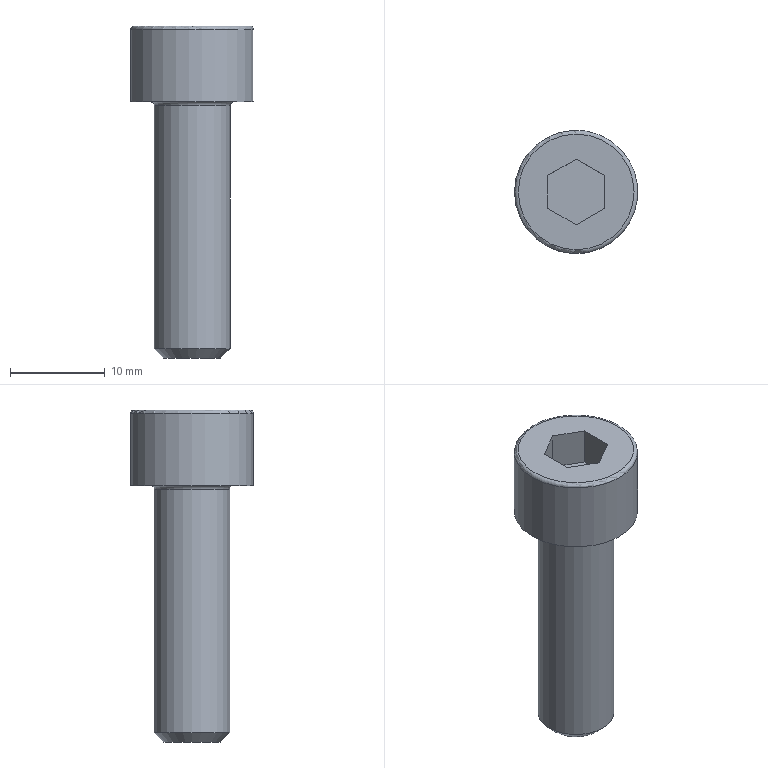Part | STEP file | solid 164 | 1 solid | 15 faces | box 13 x 13 x 35 mm | volume 2282 mm3 | plane 10 | cylinder 2 | torus 2 | cone 1 | commonest cylinder face diameters 8 x1 13 x1